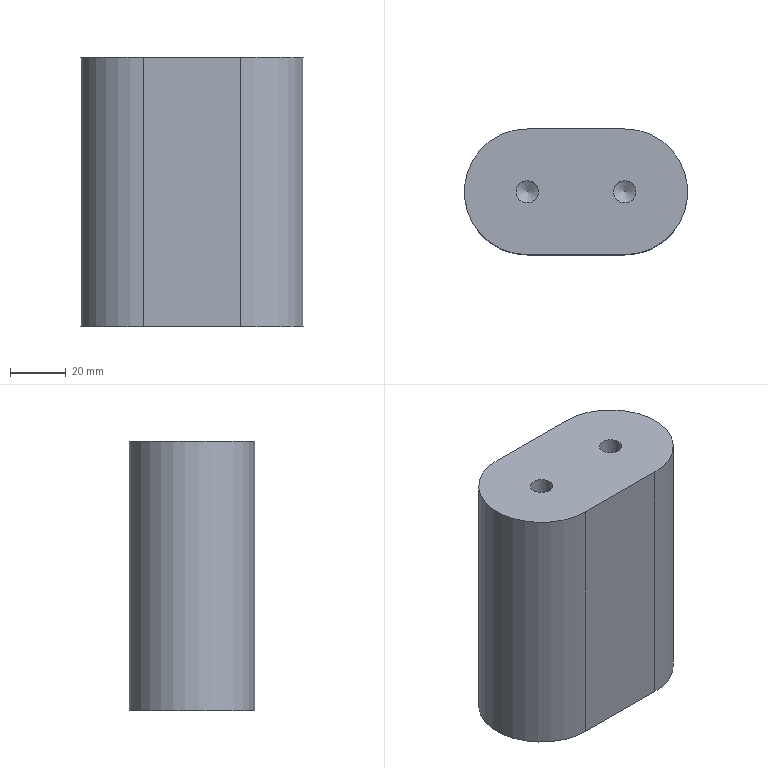Part | NX | features solid 2 | 1 solid | 10 faces | box 80.11 x 45.1 x 96.492 mm | volume 303914 mm3 | plane 4 | cylinder 4 | cone 2 | commonest cylinder face diameters 8 x2 45.1 x2
STEP:
#1=CARTESIAN_POINT('',(-302.055,793.26,83.508));
#2=VERTEX_POINT('',#1);
#3=CARTESIAN_POINT('',(-267.044,793.26,83.508));
#4=VERTEX_POINT('',#3);
#5=CARTESIAN_POINT('',(-302.055,793.26,83.508));
#6=DIRECTION('',(1.,0.,0.));
#7=VECTOR('',#6,1000.);
#8=LINE('',#5,#7);
#9=EDGE_CURVE('',#2,#4,#8,.T.);
#10=ORIENTED_EDGE('',*,*,#9,.F.);
#11=CARTESIAN_POINT('',(-302.055,793.26,180.));
#12=VERTEX_POINT('',#11);
#13=CARTESIAN_POINT('',(-302.055,793.26,200.));
#14=DIRECTION('',(0.,0.,-1.));
#15=VECTOR('',#14,1000.);
#16=LINE('',#13,#15);
#17=EDGE_CURVE('',#12,#2,#16,.T.);
#18=ORIENTED_EDGE('',*,*,#17,.F.);
#19=CARTESIAN_POINT('',(-267.044,793.26,180.));
#20=VERTEX_POINT('',#19);
#21=CARTESIAN_POINT('',(-302.055,793.26,180.));
#22=DIRECTION('',(1.,0.,0.));
#23=VECTOR('',#22,1000.);
#24=LINE('',#21,#23);
#25=EDGE_CURVE('',#12,#20,#24,.T.);
#26=ORIENTED_EDGE('',*,*,#25,.T.);
#27=CARTESIAN_POINT('',(-267.044,793.26,200.));
#28=DIRECTION('',(0.,0.,-1.));
#29=VECTOR('',#28,1000.);
#30=LINE('',#27,#29);
#31=EDGE_CURVE('',#20,#4,#30,.T.);
#32=ORIENTED_EDGE('',*,*,#31,.T.);
#33=EDGE_LOOP('',(#10,#18,#26,#32));
#34=FACE_BOUND('',#33,.T.);
#35=CARTESIAN_POINT('',(-302.055,793.26,200.));
#36=DIRECTION('',(0.,1.,0.));
#37=DIRECTION('',(0.,0.,1.));
#38=AXIS2_PLACEMENT_3D('',#35,#36,#37);
#39=PLANE('',#38);
#40=ADVANCED_FACE('',(#34),#39,.T.);
#41=CARTESIAN_POINT('',(-267.044,748.16,83.508));
#42=VERTEX_POINT('',#41);
#43=CARTESIAN_POINT('',(-302.055,748.16,83.508));
#44=VERTEX_POINT('',#43);
#45=CARTESIAN_POINT('',(-267.044,748.16,83.508));
#46=DIRECTION('',(-1.,0.,0.));
#47=VECTOR('',#46,1000.);
#48=LINE('',#45,#47);
#49=EDGE_CURVE('',#42,#44,#48,.T.);
#50=ORIENTED_EDGE('',*,*,#49,.F.);
#51=CARTESIAN_POINT('',(-267.044,748.16,180.));
#52=VERTEX_POINT('',#51);
#53=CARTESIAN_POINT('',(-267.044,748.16,200.));
#54=DIRECTION('',(0.,0.,-1.));
#55=VECTOR('',#54,1000.);
#56=LINE('',#53,#55);
#57=EDGE_CURVE('',#52,#42,#56,.T.);
#58=ORIENTED_EDGE('',*,*,#57,.F.);
#59=CARTESIAN_POINT('',(-302.055,748.16,180.));
#60=VERTEX_POINT('',#59);
#61=CARTESIAN_POINT('',(-267.044,748.16,180.));
#62=DIRECTION('',(-1.,0.,0.));
#63=VECTOR('',#62,1000.);
#64=LINE('',#61,#63);
#65=EDGE_CURVE('',#52,#60,#64,.T.);
#66=ORIENTED_EDGE('',*,*,#65,.T.);
#67=CARTESIAN_POINT('',(-302.055,748.16,200.));
#68=DIRECTION('',(0.,0.,-1.));
#69=VECTOR('',#68,1000.);
#70=LINE('',#67,#69);
#71=EDGE_CURVE('',#60,#44,#70,.T.);
#72=ORIENTED_EDGE('',*,*,#71,.T.);
#73=EDGE_LOOP('',(#50,#58,#66,#72));
#74=FACE_BOUND('',#73,.T.);
#75=CARTESIAN_POINT('',(-267.044,748.16,200.));
#76=DIRECTION('',(0.,-1.,0.));
#77=DIRECTION('',(0.,0.,-1.));
#78=AXIS2_PLACEMENT_3D('',#75,#76,#77);
#79=PLANE('',#78);
#80=ADVANCED_FACE('',(#74),#79,.T.);
#81=CARTESIAN_POINT('',(-267.044,770.71,83.508));
#82=DIRECTION('',(0.,0.,1.));
#83=DIRECTION('',(0.,-1.,0.));
#84=AXIS2_PLACEMENT_3D('',#81,#82,#83);
#85=CIRCLE('',#84,22.55);
#86=EDGE_CURVE('',#42,#4,#85,.T.);
#87=ORIENTED_EDGE('',*,*,#86,.T.);
#88=ORIENTED_EDGE('',*,*,#31,.F.);
#89=CARTESIAN_POINT('',(-267.044,770.71,180.));
#90=DIRECTION('',(0.,0.,1.));
#91=DIRECTION('',(0.,-1.,0.));
#92=AXIS2_PLACEMENT_3D('',#89,#90,#91);
#93=CIRCLE('',#92,22.55);
#94=EDGE_CURVE('',#52,#20,#93,.T.);
#95=ORIENTED_EDGE('',*,*,#94,.F.);
#96=ORIENTED_EDGE('',*,*,#57,.T.);
#97=EDGE_LOOP('',(#87,#88,#95,#96));
#98=FACE_BOUND('',#97,.T.);
#99=CARTESIAN_POINT('',(-267.044,770.71,200.));
#100=DIRECTION('',(0.,0.,-1.));
#101=DIRECTION('',(0.,1.,0.));
#102=AXIS2_PLACEMENT_3D('',#99,#100,#101);
#103=CYLINDRICAL_SURFACE('',#102,22.55);
#104=ADVANCED_FACE('',(#98),#103,.T.);
#105=CARTESIAN_POINT('',(-302.055,770.71,83.508));
#106=DIRECTION('',(0.,0.,1.));
#107=DIRECTION('',(0.,-1.,0.));
#108=AXIS2_PLACEMENT_3D('',#105,#106,#107);
#109=CIRCLE('',#108,22.55);
#110=EDGE_CURVE('',#2,#44,#109,.T.);
#111=ORIENTED_EDGE('',*,*,#110,.T.);
#112=ORIENTED_EDGE('',*,*,#71,.F.);
#113=CARTESIAN_POINT('',(-302.055,770.71,180.));
#114=DIRECTION('',(0.,0.,1.));
#115=DIRECTION('',(0.,-1.,0.));
#116=AXIS2_PLACEMENT_3D('',#113,#114,#115);
#117=CIRCLE('',#116,22.55);
#118=EDGE_CURVE('',#12,#60,#117,.T.);
#119=ORIENTED_EDGE('',*,*,#118,.F.);
#120=ORIENTED_EDGE('',*,*,#17,.T.);
#121=EDGE_LOOP('',(#111,#112,#119,#120));
#122=FACE_BOUND('',#121,.T.);
#123=CARTESIAN_POINT('',(-302.055,770.71,200.));
#124=DIRECTION('',(0.,0.,-1.));
#125=DIRECTION('',(0.,1.,0.));
#126=AXIS2_PLACEMENT_3D('',#123,#124,#125);
#127=CYLINDRICAL_SURFACE('',#126,22.55);
#128=ADVANCED_FACE('',(#122),#127,.T.);
#129=CARTESIAN_POINT('',(-271.044,770.71,180.));
#130=VERTEX_POINT('',#129);
#131=CARTESIAN_POINT('',(-267.044,770.71,180.));
#132=DIRECTION('',(0.,0.,-1.));
#133=DIRECTION('',(-1.,0.,0.));
#134=AXIS2_PLACEMENT_3D('',#131,#132,#133);
#135=CIRCLE('',#134,4.);
#136=EDGE_CURVE('',#130,#130,#135,.T.);
#137=ORIENTED_EDGE('',*,*,#136,.T.);
#138=EDGE_LOOP('',(#137));
#139=FACE_BOUND('',#138,.T.);
#140=CARTESIAN_POINT('',(-306.055,770.71,180.));
#141=VERTEX_POINT('',#140);
#142=CARTESIAN_POINT('',(-302.055,770.71,180.));
#143=DIRECTION('',(0.,0.,-1.));
#144=DIRECTION('',(-1.,0.,0.));
#145=AXIS2_PLACEMENT_3D('',#142,#143,#144);
#146=CIRCLE('',#145,4.);
#147=EDGE_CURVE('',#141,#141,#146,.T.);
#148=ORIENTED_EDGE('',*,*,#147,.T.);
#149=EDGE_LOOP('',(#148));
#150=FACE_BOUND('',#149,.T.);
#151=ORIENTED_EDGE('',*,*,#94,.T.);
#152=ORIENTED_EDGE('',*,*,#25,.F.);
#153=ORIENTED_EDGE('',*,*,#118,.T.);
#154=ORIENTED_EDGE('',*,*,#65,.F.);
#155=EDGE_LOOP('',(#151,#152,#153,#154));
#156=FACE_BOUND('',#155,.T.);
#157=CARTESIAN_POINT('',(-267.044,770.71,180.));
#158=DIRECTION('',(0.,0.,1.));
#159=DIRECTION('',(0.,-1.,0.));
#160=AXIS2_PLACEMENT_3D('',#157,#158,#159);
#161=PLANE('',#160);
#162=ADVANCED_FACE('',(#139,#150,#156),#161,.T.);
#163=ORIENTED_EDGE('',*,*,#86,.F.);
#164=ORIENTED_EDGE('',*,*,#49,.T.);
#165=ORIENTED_EDGE('',*,*,#110,.F.);
#166=ORIENTED_EDGE('',*,*,#9,.T.);
#167=EDGE_LOOP('',(#163,#164,#165,#166));
#168=FACE_BOUND('',#167,.T.);
#169=CARTESIAN_POINT('',(-267.044,770.71,83.508));
#170=DIRECTION('',(0.,0.,1.));
#171=DIRECTION('',(0.,-1.,0.));
#172=AXIS2_PLACEMENT_3D('',#169,#170,#171);
#173=PLANE('',#172);
#174=ADVANCED_FACE('',(#168),#173,.F.);
#175=CARTESIAN_POINT('',(-306.055,770.71,155.));
#176=VERTEX_POINT('',#175);
#177=CARTESIAN_POINT('',(-302.055,770.71,155.));
#178=DIRECTION('',(0.,0.,-1.));
#179=DIRECTION('',(-1.,0.,0.));
#180=AXIS2_PLACEMENT_3D('',#177,#178,#179);
#181=CIRCLE('',#180,4.);
#182=EDGE_CURVE('',#176,#176,#181,.T.);
#183=ORIENTED_EDGE('',*,*,#182,.F.);
#184=EDGE_LOOP('',(#183));
#185=FACE_BOUND('',#184,.T.);
#186=CARTESIAN_POINT('',(-302.055,770.71,152.691));
#187=VERTEX_POINT('',#186);
#188=VERTEX_LOOP('',#187);
#189=FACE_BOUND('',#188,.T.);
#190=CARTESIAN_POINT('',(-302.055,770.71,155.));
#191=DIRECTION('',(0.,0.,1.));
#192=DIRECTION('',(1.,0.,0.));
#193=AXIS2_PLACEMENT_3D('',#190,#191,#192);
#194=CONICAL_SURFACE('',#193,4.,1.047);
#195=ADVANCED_FACE('',(#185,#189),#194,.F.);
#196=ORIENTED_EDGE('',*,*,#182,.T.);
#197=EDGE_LOOP('',(#196));
#198=FACE_BOUND('',#197,.T.);
#199=ORIENTED_EDGE('',*,*,#147,.F.);
#200=EDGE_LOOP('',(#199));
#201=FACE_BOUND('',#200,.T.);
#202=CARTESIAN_POINT('',(-302.055,770.71,180.));
#203=DIRECTION('',(0.,0.,-1.));
#204=DIRECTION('',(-1.,0.,0.));
#205=AXIS2_PLACEMENT_3D('',#202,#203,#204);
#206=CYLINDRICAL_SURFACE('',#205,4.);
#207=ADVANCED_FACE('',(#198,#201),#206,.F.);
#208=CARTESIAN_POINT('',(-271.044,770.71,155.));
#209=VERTEX_POINT('',#208);
#210=CARTESIAN_POINT('',(-267.044,770.71,155.));
#211=DIRECTION('',(0.,0.,-1.));
#212=DIRECTION('',(-1.,0.,0.));
#213=AXIS2_PLACEMENT_3D('',#210,#211,#212);
#214=CIRCLE('',#213,4.);
#215=EDGE_CURVE('',#209,#209,#214,.T.);
#216=ORIENTED_EDGE('',*,*,#215,.F.);
#217=EDGE_LOOP('',(#216));
#218=FACE_BOUND('',#217,.T.);
#219=CARTESIAN_POINT('',(-267.044,770.71,152.691));
#220=VERTEX_POINT('',#219);
#221=VERTEX_LOOP('',#220);
#222=FACE_BOUND('',#221,.T.);
#223=CARTESIAN_POINT('',(-267.044,770.71,155.));
#224=DIRECTION('',(0.,0.,1.));
#225=DIRECTION('',(1.,0.,0.));
#226=AXIS2_PLACEMENT_3D('',#223,#224,#225);
#227=CONICAL_SURFACE('',#226,4.,1.047);
#228=ADVANCED_FACE('',(#218,#222),#227,.F.);
#229=ORIENTED_EDGE('',*,*,#215,.T.);
#230=EDGE_LOOP('',(#229));
#231=FACE_BOUND('',#230,.T.);
#232=ORIENTED_EDGE('',*,*,#136,.F.);
#233=EDGE_LOOP('',(#232));
#234=FACE_BOUND('',#233,.T.);
#235=CARTESIAN_POINT('',(-267.044,770.71,180.));
#236=DIRECTION('',(0.,0.,-1.));
#237=DIRECTION('',(-1.,0.,0.));
#238=AXIS2_PLACEMENT_3D('',#235,#236,#237);
#239=CYLINDRICAL_SURFACE('',#238,4.);
#240=ADVANCED_FACE('',(#231,#234),#239,.F.);
#241=CLOSED_SHELL('',(#40,#80,#104,#128,#162,#174,#195,#207,#228,#240));
#242=MANIFOLD_SOLID_BREP('',#241);
#243=(LENGTH_UNIT()NAMED_UNIT(*)SI_UNIT(.MILLI.,.METRE.));
#244=UNCERTAINTY_MEASURE_WITH_UNIT(LENGTH_MEASURE(0.00001),#243,'','');
#245=(NAMED_UNIT(*)PLANE_ANGLE_UNIT()SI_UNIT($,.RADIAN.));
#246=(NAMED_UNIT(*)SI_UNIT($,.STERADIAN.)SOLID_ANGLE_UNIT());
#247=(GEOMETRIC_REPRESENTATION_CONTEXT(3)GLOBAL_UNCERTAINTY_ASSIGNED_CONTEXT((#244))GLOBAL_UNIT_ASSIGNED_CONTEXT((#243,#245,#246))REPRESENTATION_CONTEXT('',''));
#248=ADVANCED_BREP_SHAPE_REPRESENTATION('',(#242),#247);